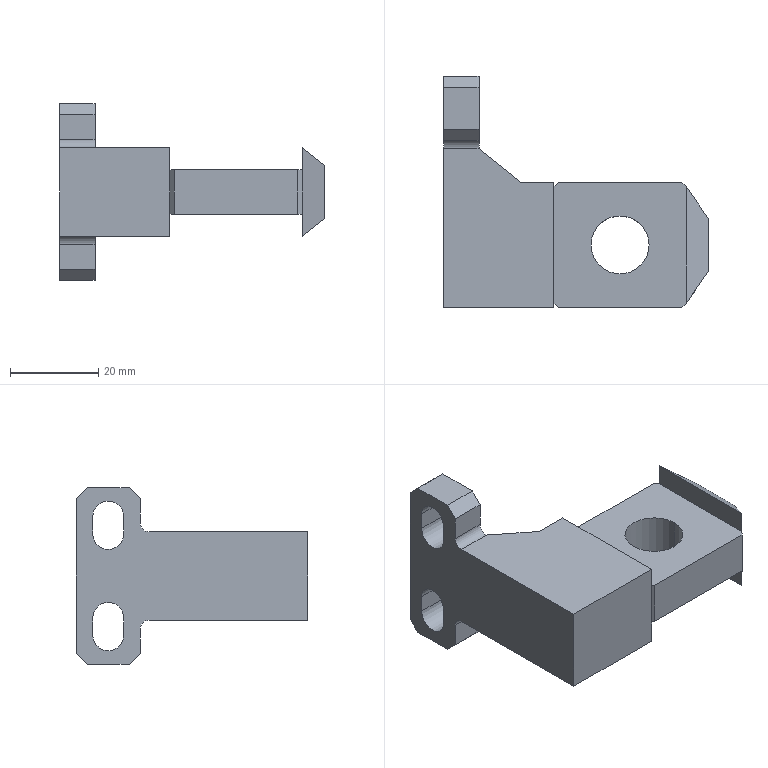Part | SolidWorks | features BaseBody 1 | 1 solid | 52 faces | box 60 x 52.5 x 40 mm | volume 28461 mm3 | plane 38 | cylinder 14 | commonest cylinder face diameters 7 x6 4 x2 6 x2 8 x2 13.157 x2
STEP:
#1=CARTESIAN_POINT('',(-6.579,0.,-5.));
#2=VERTEX_POINT('',#1);
#3=CARTESIAN_POINT('',(6.579,0.,-5.));
#4=VERTEX_POINT('',#3);
#5=CARTESIAN_POINT('',(0.,0.,-5.));
#6=DIRECTION('',(0.,0.,-1.));
#7=DIRECTION('',(-1.,0.,0.));
#8=AXIS2_PLACEMENT_3D('',#5,#6,#7);
#9=CIRCLE('',#8,6.579);
#10=EDGE_CURVE('',#2,#4,#9,.T.);
#11=ORIENTED_EDGE('',*,*,#10,.T.);
#12=CARTESIAN_POINT('',(6.579,0.,5.));
#13=VERTEX_POINT('',#12);
#14=CARTESIAN_POINT('',(6.579,0.,-5.));
#15=DIRECTION('',(0.,0.,1.));
#16=VECTOR('',#15,1000.);
#17=LINE('',#14,#16);
#18=EDGE_CURVE('',#4,#13,#17,.T.);
#19=ORIENTED_EDGE('',*,*,#18,.T.);
#20=CARTESIAN_POINT('',(-6.579,0.,5.));
#21=VERTEX_POINT('',#20);
#22=CARTESIAN_POINT('',(0.,0.,5.));
#23=DIRECTION('',(0.,0.,-1.));
#24=DIRECTION('',(-1.,0.,0.));
#25=AXIS2_PLACEMENT_3D('',#22,#23,#24);
#26=CIRCLE('',#25,6.579);
#27=EDGE_CURVE('',#21,#13,#26,.T.);
#28=ORIENTED_EDGE('',*,*,#27,.F.);
#29=CARTESIAN_POINT('',(-6.579,0.,-5.));
#30=DIRECTION('',(0.,0.,1.));
#31=VECTOR('',#30,1000.);
#32=LINE('',#29,#31);
#33=EDGE_CURVE('',#2,#21,#32,.T.);
#34=ORIENTED_EDGE('',*,*,#33,.F.);
#35=EDGE_LOOP('',(#11,#19,#28,#34));
#36=FACE_OUTER_BOUND('',#35,.T.);
#37=CARTESIAN_POINT('',(0.,0.,-5.));
#38=DIRECTION('',(0.,0.,1.));
#39=DIRECTION('',(-1.,0.,0.));
#40=AXIS2_PLACEMENT_3D('',#37,#38,#39);
#41=CYLINDRICAL_SURFACE('',#40,6.579);
#42=ADVANCED_FACE('',(#36),#41,.F.);
#43=CARTESIAN_POINT('',(20.,0.,-4.));
#44=VERTEX_POINT('',#43);
#45=CARTESIAN_POINT('',(20.,0.,4.));
#46=VERTEX_POINT('',#45);
#47=CARTESIAN_POINT('',(20.,0.,0.));
#48=DIRECTION('',(1.,0.,0.));
#49=DIRECTION('',(0.,0.,-1.));
#50=AXIS2_PLACEMENT_3D('',#47,#48,#49);
#51=CIRCLE('',#50,4.);
#52=EDGE_CURVE('',#44,#46,#51,.T.);
#53=ORIENTED_EDGE('',*,*,#52,.T.);
#54=CARTESIAN_POINT('',(18.,0.,4.));
#55=VERTEX_POINT('',#54);
#56=CARTESIAN_POINT('',(20.,0.,4.));
#57=DIRECTION('',(-1.,0.,0.));
#58=VECTOR('',#57,1000.);
#59=LINE('',#56,#58);
#60=EDGE_CURVE('',#46,#55,#59,.T.);
#61=ORIENTED_EDGE('',*,*,#60,.T.);
#62=CARTESIAN_POINT('',(18.,0.,-4.));
#63=VERTEX_POINT('',#62);
#64=CARTESIAN_POINT('',(18.,0.,0.));
#65=DIRECTION('',(1.,0.,0.));
#66=DIRECTION('',(0.,0.,-1.));
#67=AXIS2_PLACEMENT_3D('',#64,#65,#66);
#68=CIRCLE('',#67,4.);
#69=EDGE_CURVE('',#63,#55,#68,.T.);
#70=ORIENTED_EDGE('',*,*,#69,.F.);
#71=CARTESIAN_POINT('',(20.,0.,-4.));
#72=DIRECTION('',(-1.,0.,0.));
#73=VECTOR('',#72,1000.);
#74=LINE('',#71,#73);
#75=EDGE_CURVE('',#44,#63,#74,.T.);
#76=ORIENTED_EDGE('',*,*,#75,.F.);
#77=EDGE_LOOP('',(#53,#61,#70,#76));
#78=FACE_OUTER_BOUND('',#77,.T.);
#79=CARTESIAN_POINT('',(20.,0.,0.));
#80=DIRECTION('',(-1.,0.,0.));
#81=DIRECTION('',(0.,0.,-1.));
#82=AXIS2_PLACEMENT_3D('',#79,#80,#81);
#83=CYLINDRICAL_SURFACE('',#82,4.);
#84=ADVANCED_FACE('',(#78),#83,.F.);
#85=CARTESIAN_POINT('',(18.,0.,-3.));
#86=VERTEX_POINT('',#85);
#87=CARTESIAN_POINT('',(18.,0.,3.));
#88=VERTEX_POINT('',#87);
#89=CARTESIAN_POINT('',(18.,0.,0.));
#90=DIRECTION('',(1.,0.,0.));
#91=DIRECTION('',(0.,0.,-1.));
#92=AXIS2_PLACEMENT_3D('',#89,#90,#91);
#93=CIRCLE('',#92,3.);
#94=EDGE_CURVE('',#86,#88,#93,.T.);
#95=ORIENTED_EDGE('',*,*,#94,.T.);
#96=CARTESIAN_POINT('',(12.,0.,3.));
#97=VERTEX_POINT('',#96);
#98=CARTESIAN_POINT('',(20.,0.,3.));
#99=DIRECTION('',(-1.,0.,0.));
#100=VECTOR('',#99,1000.);
#101=LINE('',#98,#100);
#102=EDGE_CURVE('',#88,#97,#101,.T.);
#103=ORIENTED_EDGE('',*,*,#102,.T.);
#104=CARTESIAN_POINT('',(12.,0.,-3.));
#105=VERTEX_POINT('',#104);
#106=CARTESIAN_POINT('',(12.,0.,0.));
#107=DIRECTION('',(1.,0.,0.));
#108=DIRECTION('',(0.,0.,-1.));
#109=AXIS2_PLACEMENT_3D('',#106,#107,#108);
#110=CIRCLE('',#109,3.);
#111=EDGE_CURVE('',#105,#97,#110,.T.);
#112=ORIENTED_EDGE('',*,*,#111,.F.);
#113=CARTESIAN_POINT('',(20.,0.,-3.));
#114=DIRECTION('',(-1.,0.,0.));
#115=VECTOR('',#114,1000.);
#116=LINE('',#113,#115);
#117=EDGE_CURVE('',#86,#105,#116,.T.);
#118=ORIENTED_EDGE('',*,*,#117,.F.);
#119=EDGE_LOOP('',(#95,#103,#112,#118));
#120=FACE_OUTER_BOUND('',#119,.T.);
#121=CARTESIAN_POINT('',(20.,0.,0.));
#122=DIRECTION('',(-1.,0.,0.));
#123=DIRECTION('',(0.,0.,-1.));
#124=AXIS2_PLACEMENT_3D('',#121,#122,#123);
#125=CYLINDRICAL_SURFACE('',#124,3.);
#126=ADVANCED_FACE('',(#120),#125,.F.);
#127=CARTESIAN_POINT('',(-40.,31.,-6.));
#128=VERTEX_POINT('',#127);
#129=CARTESIAN_POINT('',(-40.,27.5,-9.5));
#130=VERTEX_POINT('',#129);
#131=CARTESIAN_POINT('',(-40.,31.,-9.5));
#132=DIRECTION('',(1.,0.,0.));
#133=DIRECTION('',(0.,0.,-1.));
#134=AXIS2_PLACEMENT_3D('',#131,#132,#133);
#135=CIRCLE('',#134,3.5);
#136=EDGE_CURVE('',#128,#130,#135,.T.);
#137=ORIENTED_EDGE('',*,*,#136,.F.);
#138=CARTESIAN_POINT('',(-32.,31.,-6.));
#139=VERTEX_POINT('',#138);
#140=CARTESIAN_POINT('',(-32.,31.,-6.));
#141=DIRECTION('',(1.,0.,0.));
#142=VECTOR('',#141,1000.);
#143=LINE('',#140,#142);
#144=EDGE_CURVE('',#128,#139,#143,.T.);
#145=ORIENTED_EDGE('',*,*,#144,.T.);
#146=CARTESIAN_POINT('',(-32.,27.5,-9.5));
#147=VERTEX_POINT('',#146);
#148=CARTESIAN_POINT('',(-32.,31.,-9.5));
#149=DIRECTION('',(1.,0.,0.));
#150=DIRECTION('',(0.,0.,-1.));
#151=AXIS2_PLACEMENT_3D('',#148,#149,#150);
#152=CIRCLE('',#151,3.5);
#153=EDGE_CURVE('',#139,#147,#152,.T.);
#154=ORIENTED_EDGE('',*,*,#153,.T.);
#155=CARTESIAN_POINT('',(-32.,27.5,-9.5));
#156=DIRECTION('',(-1.,0.,0.));
#157=VECTOR('',#156,1000.);
#158=LINE('',#155,#157);
#159=EDGE_CURVE('',#147,#130,#158,.T.);
#160=ORIENTED_EDGE('',*,*,#159,.T.);
#161=EDGE_LOOP('',(#137,#145,#154,#160));
#162=FACE_OUTER_BOUND('',#161,.T.);
#163=CARTESIAN_POINT('',(-32.,31.,-9.5));
#164=DIRECTION('',(1.,0.,0.));
#165=DIRECTION('',(0.,0.,1.));
#166=AXIS2_PLACEMENT_3D('',#163,#164,#165);
#167=CYLINDRICAL_SURFACE('',#166,3.5);
#168=ADVANCED_FACE('',(#162),#167,.F.);
#169=CARTESIAN_POINT('',(-40.,31.,17.));
#170=VERTEX_POINT('',#169);
#171=CARTESIAN_POINT('',(-40.,27.5,13.5));
#172=VERTEX_POINT('',#171);
#173=CARTESIAN_POINT('',(-40.,31.,13.5));
#174=DIRECTION('',(1.,0.,0.));
#175=DIRECTION('',(0.,0.,-1.));
#176=AXIS2_PLACEMENT_3D('',#173,#174,#175);
#177=CIRCLE('',#176,3.5);
#178=EDGE_CURVE('',#170,#172,#177,.T.);
#179=ORIENTED_EDGE('',*,*,#178,.F.);
#180=CARTESIAN_POINT('',(-32.,31.,17.));
#181=VERTEX_POINT('',#180);
#182=CARTESIAN_POINT('',(-32.,31.,17.));
#183=DIRECTION('',(1.,0.,0.));
#184=VECTOR('',#183,1000.);
#185=LINE('',#182,#184);
#186=EDGE_CURVE('',#170,#181,#185,.T.);
#187=ORIENTED_EDGE('',*,*,#186,.T.);
#188=CARTESIAN_POINT('',(-32.,27.5,13.5));
#189=VERTEX_POINT('',#188);
#190=CARTESIAN_POINT('',(-32.,31.,13.5));
#191=DIRECTION('',(1.,0.,0.));
#192=DIRECTION('',(0.,0.,-1.));
#193=AXIS2_PLACEMENT_3D('',#190,#191,#192);
#194=CIRCLE('',#193,3.5);
#195=EDGE_CURVE('',#181,#189,#194,.T.);
#196=ORIENTED_EDGE('',*,*,#195,.T.);
#197=CARTESIAN_POINT('',(-32.,27.5,13.5));
#198=DIRECTION('',(-1.,0.,0.));
#199=VECTOR('',#198,1000.);
#200=LINE('',#197,#199);
#201=EDGE_CURVE('',#189,#172,#200,.T.);
#202=ORIENTED_EDGE('',*,*,#201,.T.);
#203=EDGE_LOOP('',(#179,#187,#196,#202));
#204=FACE_OUTER_BOUND('',#203,.T.);
#205=CARTESIAN_POINT('',(-32.,31.,13.5));
#206=DIRECTION('',(1.,0.,0.));
#207=DIRECTION('',(0.,0.,1.));
#208=AXIS2_PLACEMENT_3D('',#205,#206,#207);
#209=CYLINDRICAL_SURFACE('',#208,3.5);
#210=ADVANCED_FACE('',(#204),#209,.F.);
#211=CARTESIAN_POINT('',(15.,13.25,-10.));
#212=VERTEX_POINT('',#211);
#213=CARTESIAN_POINT('',(20.,6.,-6.));
#214=VERTEX_POINT('',#213);
#215=CARTESIAN_POINT('',(23.42,1.041,-3.264));
#216=DIRECTION('',(0.5169,-0.7495,0.4135));
#217=VECTOR('',#216,1000.);
#218=LINE('',#215,#217);
#219=EDGE_CURVE('',#212,#214,#218,.T.);
#220=ORIENTED_EDGE('',*,*,#219,.T.);
#221=CARTESIAN_POINT('',(20.,-6.,-6.));
#222=VERTEX_POINT('',#221);
#223=CARTESIAN_POINT('',(20.,13.25,-6.));
#224=DIRECTION('',(0.,-1.,0.));
#225=VECTOR('',#224,1000.);
#226=LINE('',#223,#225);
#227=EDGE_CURVE('',#214,#222,#226,.T.);
#228=ORIENTED_EDGE('',*,*,#227,.T.);
#229=CARTESIAN_POINT('',(15.,-13.25,-10.));
#230=VERTEX_POINT('',#229);
#231=CARTESIAN_POINT('',(19.275,-7.051,-6.58));
#232=DIRECTION('',(-0.5169,-0.7495,-0.4135));
#233=VECTOR('',#232,1000.);
#234=LINE('',#231,#233);
#235=EDGE_CURVE('',#222,#230,#234,.T.);
#236=ORIENTED_EDGE('',*,*,#235,.T.);
#237=CARTESIAN_POINT('',(15.,13.25,-10.));
#238=DIRECTION('',(0.,-1.,0.));
#239=VECTOR('',#238,1000.);
#240=LINE('',#237,#239);
#241=EDGE_CURVE('',#212,#230,#240,.T.);
#242=ORIENTED_EDGE('',*,*,#241,.F.);
#243=EDGE_LOOP('',(#220,#228,#236,#242));
#244=FACE_OUTER_BOUND('',#243,.T.);
#245=CARTESIAN_POINT('',(15.,13.25,-10.));
#246=DIRECTION('',(0.6247,0.,-0.7809));
#247=DIRECTION('',(0.,-1.,0.));
#248=AXIS2_PLACEMENT_3D('',#245,#246,#247);
#249=PLANE('',#248);
#250=ADVANCED_FACE('',(#244),#249,.T.);
#251=CARTESIAN_POINT('',(20.,6.,6.));
#252=VERTEX_POINT('',#251);
#253=CARTESIAN_POINT('',(15.,13.25,10.));
#254=VERTEX_POINT('',#253);
#255=CARTESIAN_POINT('',(19.145,7.24,6.684));
#256=DIRECTION('',(-0.5169,0.7495,0.4135));
#257=VECTOR('',#256,1000.);
#258=LINE('',#255,#257);
#259=EDGE_CURVE('',#252,#254,#258,.T.);
#260=ORIENTED_EDGE('',*,*,#259,.T.);
#261=CARTESIAN_POINT('',(15.,-13.25,10.));
#262=VERTEX_POINT('',#261);
#263=CARTESIAN_POINT('',(15.,13.25,10.));
#264=DIRECTION('',(0.,-1.,0.));
#265=VECTOR('',#264,1000.);
#266=LINE('',#263,#265);
#267=EDGE_CURVE('',#254,#262,#266,.T.);
#268=ORIENTED_EDGE('',*,*,#267,.T.);
#269=CARTESIAN_POINT('',(20.,-6.,6.));
#270=VERTEX_POINT('',#269);
#271=CARTESIAN_POINT('',(15.,-13.25,10.));
#272=DIRECTION('',(0.5169,0.7495,-0.4135));
#273=VECTOR('',#272,1000.);
#274=LINE('',#271,#273);
#275=EDGE_CURVE('',#262,#270,#274,.T.);
#276=ORIENTED_EDGE('',*,*,#275,.T.);
#277=CARTESIAN_POINT('',(20.,13.25,6.));
#278=DIRECTION('',(0.,-1.,0.));
#279=VECTOR('',#278,1000.);
#280=LINE('',#277,#279);
#281=EDGE_CURVE('',#252,#270,#280,.T.);
#282=ORIENTED_EDGE('',*,*,#281,.F.);
#283=EDGE_LOOP('',(#260,#268,#276,#282));
#284=FACE_OUTER_BOUND('',#283,.T.);
#285=CARTESIAN_POINT('',(20.,13.25,6.));
#286=DIRECTION('',(0.6247,0.,0.7809));
#287=DIRECTION('',(0.,-1.,0.));
#288=AXIS2_PLACEMENT_3D('',#285,#286,#287);
#289=PLANE('',#288);
#290=ADVANCED_FACE('',(#284),#289,.T.);
#291=CARTESIAN_POINT('',(15.,-13.25,5.));
#292=VERTEX_POINT('',#291);
#293=CARTESIAN_POINT('',(15.,13.25,5.));
#294=VERTEX_POINT('',#293);
#295=CARTESIAN_POINT('',(15.,-13.25,5.));
#296=DIRECTION('',(0.,1.,0.));
#297=VECTOR('',#296,1000.);
#298=LINE('',#295,#297);
#299=EDGE_CURVE('',#292,#294,#298,.T.);
#300=ORIENTED_EDGE('',*,*,#299,.F.);
#301=CARTESIAN_POINT('',(15.,-13.25,10.));
#302=DIRECTION('',(0.,0.,-1.));
#303=VECTOR('',#302,1000.);
#304=LINE('',#301,#303);
#305=EDGE_CURVE('',#262,#292,#304,.T.);
#306=ORIENTED_EDGE('',*,*,#305,.F.);
#307=ORIENTED_EDGE('',*,*,#267,.F.);
#308=CARTESIAN_POINT('',(15.,13.25,10.));
#309=DIRECTION('',(0.,0.,-1.));
#310=VECTOR('',#309,1000.);
#311=LINE('',#308,#310);
#312=EDGE_CURVE('',#254,#294,#311,.T.);
#313=ORIENTED_EDGE('',*,*,#312,.T.);
#314=EDGE_LOOP('',(#300,#306,#307,#313));
#315=FACE_OUTER_BOUND('',#314,.T.);
#316=CARTESIAN_POINT('',(15.,13.25,10.));
#317=DIRECTION('',(1.,0.,0.));
#318=DIRECTION('',(0.,1.,0.));
#319=AXIS2_PLACEMENT_3D('',#316,#317,#318);
#320=PLANE('',#319);
#321=ADVANCED_FACE('',(#315),#320,.F.);
#322=ORIENTED_EDGE('',*,*,#259,.F.);
#323=CARTESIAN_POINT('',(20.,6.,10.));
#324=DIRECTION('',(0.,0.,-1.));
#325=VECTOR('',#324,1000.);
#326=LINE('',#323,#325);
#327=EDGE_CURVE('',#252,#214,#326,.T.);
#328=ORIENTED_EDGE('',*,*,#327,.T.);
#329=ORIENTED_EDGE('',*,*,#219,.F.);
#330=CARTESIAN_POINT('',(15.,13.25,-5.));
#331=VERTEX_POINT('',#330);
#332=CARTESIAN_POINT('',(15.,13.25,10.));
#333=DIRECTION('',(0.,0.,-1.));
#334=VECTOR('',#333,1000.);
#335=LINE('',#332,#334);
#336=EDGE_CURVE('',#331,#212,#335,.T.);
#337=ORIENTED_EDGE('',*,*,#336,.F.);
#338=CARTESIAN_POINT('',(15.,13.25,5.));
#339=DIRECTION('',(0.,0.,-1.));
#340=VECTOR('',#339,1000.);
#341=LINE('',#338,#340);
#342=EDGE_CURVE('',#294,#331,#341,.T.);
#343=ORIENTED_EDGE('',*,*,#342,.F.);
#344=ORIENTED_EDGE('',*,*,#312,.F.);
#345=EDGE_LOOP('',(#322,#328,#329,#337,#343,#344));
#346=FACE_OUTER_BOUND('',#345,.T.);
#347=CARTESIAN_POINT('',(20.,6.,10.));
#348=DIRECTION('',(-0.8232,-0.5677,0.));
#349=DIRECTION('',(-0.5677,0.8232,0.));
#350=AXIS2_PLACEMENT_3D('',#347,#348,#349);
#351=PLANE('',#350);
#352=ADVANCED_FACE('',(#346),#351,.F.);
#353=ORIENTED_EDGE('',*,*,#275,.F.);
#354=ORIENTED_EDGE('',*,*,#305,.T.);
#355=CARTESIAN_POINT('',(15.,-13.25,-5.));
#356=VERTEX_POINT('',#355);
#357=CARTESIAN_POINT('',(15.,-13.25,5.));
#358=DIRECTION('',(0.,0.,-1.));
#359=VECTOR('',#358,1000.);
#360=LINE('',#357,#359);
#361=EDGE_CURVE('',#292,#356,#360,.T.);
#362=ORIENTED_EDGE('',*,*,#361,.T.);
#363=CARTESIAN_POINT('',(15.,-13.25,10.));
#364=DIRECTION('',(0.,0.,-1.));
#365=VECTOR('',#364,1000.);
#366=LINE('',#363,#365);
#367=EDGE_CURVE('',#356,#230,#366,.T.);
#368=ORIENTED_EDGE('',*,*,#367,.T.);
#369=ORIENTED_EDGE('',*,*,#235,.F.);
#370=CARTESIAN_POINT('',(20.,-6.,10.));
#371=DIRECTION('',(0.,0.,-1.));
#372=VECTOR('',#371,1000.);
#373=LINE('',#370,#372);
#374=EDGE_CURVE('',#270,#222,#373,.T.);
#375=ORIENTED_EDGE('',*,*,#374,.F.);
#376=EDGE_LOOP('',(#353,#354,#362,#368,#369,#375));
#377=FACE_OUTER_BOUND('',#376,.T.);
#378=CARTESIAN_POINT('',(15.,-13.25,10.));
#379=DIRECTION('',(-0.8232,0.5677,0.));
#380=DIRECTION('',(0.,0.,1.));
#381=AXIS2_PLACEMENT_3D('',#378,#379,#380);
#382=PLANE('',#381);
#383=ADVANCED_FACE('',(#377),#382,.F.);
#384=ORIENTED_EDGE('',*,*,#27,.T.);
#385=CARTESIAN_POINT('',(0.,0.,5.));
#386=DIRECTION('',(0.,0.,-1.));
#387=DIRECTION('',(-1.,0.,0.));
#388=AXIS2_PLACEMENT_3D('',#385,#386,#387);
#389=CIRCLE('',#388,6.579);
#390=EDGE_CURVE('',#13,#21,#389,.T.);
#391=ORIENTED_EDGE('',*,*,#390,.T.);
#392=EDGE_LOOP('',(#384,#391));
#393=FACE_BOUND('',#392,.T.);
#394=CARTESIAN_POINT('',(-14.,14.25,5.));
#395=VERTEX_POINT('',#394);
#396=CARTESIAN_POINT('',(-15.,13.25,5.));
#397=VERTEX_POINT('',#396);
#398=CARTESIAN_POINT('',(-14.,14.25,5.));
#399=DIRECTION('',(-0.7071,-0.7071,0.));
#400=VECTOR('',#399,1000.);
#401=LINE('',#398,#400);
#402=EDGE_CURVE('',#395,#397,#401,.T.);
#403=ORIENTED_EDGE('',*,*,#402,.T.);
#404=CARTESIAN_POINT('',(-15.,-13.25,5.));
#405=VERTEX_POINT('',#404);
#406=CARTESIAN_POINT('',(-15.,13.25,5.));
#407=DIRECTION('',(0.,-1.,0.));
#408=VECTOR('',#407,1000.);
#409=LINE('',#406,#408);
#410=EDGE_CURVE('',#397,#405,#409,.T.);
#411=ORIENTED_EDGE('',*,*,#410,.T.);
#412=CARTESIAN_POINT('',(-14.,-14.25,5.));
#413=VERTEX_POINT('',#412);
#414=CARTESIAN_POINT('',(-15.,-13.25,5.));
#415=DIRECTION('',(0.7071,-0.7071,0.));
#416=VECTOR('',#415,1000.);
#417=LINE('',#414,#416);
#418=EDGE_CURVE('',#405,#413,#417,.T.);
#419=ORIENTED_EDGE('',*,*,#418,.T.);
#420=CARTESIAN_POINT('',(14.,-14.25,5.));
#421=VERTEX_POINT('',#420);
#422=CARTESIAN_POINT('',(-14.,-14.25,5.));
#423=DIRECTION('',(1.,0.,0.));
#424=VECTOR('',#423,1000.);
#425=LINE('',#422,#424);
#426=EDGE_CURVE('',#413,#421,#425,.T.);
#427=ORIENTED_EDGE('',*,*,#426,.T.);
#428=CARTESIAN_POINT('',(14.,-14.25,5.));
#429=DIRECTION('',(0.7071,0.7071,0.));
#430=VECTOR('',#429,1000.);
#431=LINE('',#428,#430);
#432=EDGE_CURVE('',#421,#292,#431,.T.);
#433=ORIENTED_EDGE('',*,*,#432,.T.);
#434=ORIENTED_EDGE('',*,*,#299,.T.);
#435=CARTESIAN_POINT('',(14.,14.25,5.));
#436=VERTEX_POINT('',#435);
#437=CARTESIAN_POINT('',(15.,13.25,5.));
#438=DIRECTION('',(-0.7071,0.7071,0.));
#439=VECTOR('',#438,1000.);
#440=LINE('',#437,#439);
#441=EDGE_CURVE('',#294,#436,#440,.T.);
#442=ORIENTED_EDGE('',*,*,#441,.T.);
#443=CARTESIAN_POINT('',(14.,14.25,5.));
#444=DIRECTION('',(-1.,0.,0.));
#445=VECTOR('',#444,1000.);
#446=LINE('',#443,#445);
#447=EDGE_CURVE('',#436,#395,#446,.T.);
#448=ORIENTED_EDGE('',*,*,#447,.T.);
#449=EDGE_LOOP('',(#403,#411,#419,#427,#433,#434,#442,#448));
#450=FACE_OUTER_BOUND('',#449,.T.);
#451=CARTESIAN_POINT('',(0.,0.,5.));
#452=DIRECTION('',(0.,0.,1.));
#453=DIRECTION('',(1.,0.,0.));
#454=AXIS2_PLACEMENT_3D('',#451,#452,#453);
#455=PLANE('',#454);
#456=ADVANCED_FACE('',(#393,#450),#455,.T.);
#457=ORIENTED_EDGE('',*,*,#10,.F.);
#458=CARTESIAN_POINT('',(0.,0.,-5.));
#459=DIRECTION('',(0.,0.,-1.));
#460=DIRECTION('',(-1.,0.,0.));
#461=AXIS2_PLACEMENT_3D('',#458,#459,#460);
#462=CIRCLE('',#461,6.579);
#463=EDGE_CURVE('',#4,#2,#462,.T.);
#464=ORIENTED_EDGE('',*,*,#463,.F.);
#465=EDGE_LOOP('',(#457,#464));
#466=FACE_BOUND('',#465,.T.);
#467=CARTESIAN_POINT('',(-14.,14.25,-5.));
#468=VERTEX_POINT('',#467);
#469=CARTESIAN_POINT('',(-15.,13.25,-5.));
#470=VERTEX_POINT('',#469);
#471=CARTESIAN_POINT('',(-14.,14.25,-5.));
#472=DIRECTION('',(-0.7071,-0.7071,0.));
#473=VECTOR('',#472,1000.);
#474=LINE('',#471,#473);
#475=EDGE_CURVE('',#468,#470,#474,.T.);
#476=ORIENTED_EDGE('',*,*,#475,.F.);
#477=CARTESIAN_POINT('',(14.,14.25,-5.));
#478=VERTEX_POINT('',#477);
#479=CARTESIAN_POINT('',(14.,14.25,-5.));
#480=DIRECTION('',(-1.,0.,0.));
#481=VECTOR('',#480,1000.);
#482=LINE('',#479,#481);
#483=EDGE_CURVE('',#478,#468,#482,.T.);
#484=ORIENTED_EDGE('',*,*,#483,.F.);
#485=CARTESIAN_POINT('',(15.,13.25,-5.));
#486=DIRECTION('',(-0.7071,0.7071,0.));
#487=VECTOR('',#486,1000.);
#488=LINE('',#485,#487);
#489=EDGE_CURVE('',#331,#478,#488,.T.);
#490=ORIENTED_EDGE('',*,*,#489,.F.);
#491=CARTESIAN_POINT('',(15.,-13.25,-5.));
#492=DIRECTION('',(0.,1.,0.));
#493=VECTOR('',#492,1000.);
#494=LINE('',#491,#493);
#495=EDGE_CURVE('',#356,#331,#494,.T.);
#496=ORIENTED_EDGE('',*,*,#495,.F.);
#497=CARTESIAN_POINT('',(14.,-14.25,-5.));
#498=VERTEX_POINT('',#497);
#499=CARTESIAN_POINT('',(14.,-14.25,-5.));
#500=DIRECTION('',(0.7071,0.7071,0.));
#501=VECTOR('',#500,1000.);
#502=LINE('',#499,#501);
#503=EDGE_CURVE('',#498,#356,#502,.T.);
#504=ORIENTED_EDGE('',*,*,#503,.F.);
#505=CARTESIAN_POINT('',(-14.,-14.25,-5.));
#506=VERTEX_POINT('',#505);
#507=CARTESIAN_POINT('',(-14.,-14.25,-5.));
#508=DIRECTION('',(1.,0.,0.));
#509=VECTOR('',#508,1000.);
#510=LINE('',#507,#509);
#511=EDGE_CURVE('',#506,#498,#510,.T.);
#512=ORIENTED_EDGE('',*,*,#511,.F.);
#513=CARTESIAN_POINT('',(-15.,-13.25,-5.));
#514=VERTEX_POINT('',#513);
#515=CARTESIAN_POINT('',(-15.,-13.25,-5.));
#516=DIRECTION('',(0.7071,-0.7071,0.));
#517=VECTOR('',#516,1000.);
#518=LINE('',#515,#517);
#519=EDGE_CURVE('',#514,#506,#518,.T.);
#520=ORIENTED_EDGE('',*,*,#519,.F.);
#521=CARTESIAN_POINT('',(-15.,13.25,-5.));
#522=DIRECTION('',(0.,-1.,0.));
#523=VECTOR('',#522,1000.);
#524=LINE('',#521,#523);
#525=EDGE_CURVE('',#470,#514,#524,.T.);
#526=ORIENTED_EDGE('',*,*,#525,.F.);
#527=EDGE_LOOP('',(#476,#484,#490,#496,#504,#512,#520,#526));
#528=FACE_OUTER_BOUND('',#527,.T.);
#529=CARTESIAN_POINT('',(0.,0.,-5.));
#530=DIRECTION('',(0.,0.,1.));
#531=DIRECTION('',(1.,0.,0.));
#532=AXIS2_PLACEMENT_3D('',#529,#530,#531);
#533=PLANE('',#532);
#534=ADVANCED_FACE('',(#466,#528),#533,.F.);
#535=ORIENTED_EDGE('',*,*,#483,.T.);
#536=CARTESIAN_POINT('',(-14.,14.25,5.));
#537=DIRECTION('',(0.,0.,-1.));
#538=VECTOR('',#537,1000.);
#539=LINE('',#536,#538);
#540=EDGE_CURVE('',#395,#468,#539,.T.);
#541=ORIENTED_EDGE('',*,*,#540,.F.);
#542=ORIENTED_EDGE('',*,*,#447,.F.);
#543=CARTESIAN_POINT('',(14.,14.25,5.));
#544=DIRECTION('',(0.,0.,-1.));
#545=VECTOR('',#544,1000.);
#546=LINE('',#543,#545);
#547=EDGE_CURVE('',#436,#478,#546,.T.);
#548=ORIENTED_EDGE('',*,*,#547,.T.);
#549=EDGE_LOOP('',(#535,#541,#542,#548));
#550=FACE_OUTER_BOUND('',#549,.T.);
#551=CARTESIAN_POINT('',(14.,14.25,5.));
#552=DIRECTION('',(0.,-1.,0.));
#553=DIRECTION('',(0.,0.,-1.));
#554=AXIS2_PLACEMENT_3D('',#551,#552,#553);
#555=PLANE('',#554);
#556=ADVANCED_FACE('',(#550),#555,.F.);
#557=ORIENTED_EDGE('',*,*,#489,.T.);
#558=ORIENTED_EDGE('',*,*,#547,.F.);
#559=ORIENTED_EDGE('',*,*,#441,.F.);
#560=ORIENTED_EDGE('',*,*,#342,.T.);
#561=EDGE_LOOP('',(#557,#558,#559,#560));
#562=FACE_OUTER_BOUND('',#561,.T.);
#563=CARTESIAN_POINT('',(15.,13.25,5.));
#564=DIRECTION('',(-0.7071,-0.7071,0.));
#565=DIRECTION('',(-0.7071,0.7071,0.));
#566=AXIS2_PLACEMENT_3D('',#563,#564,#565);
#567=PLANE('',#566);
#568=ADVANCED_FACE('',(#562),#567,.F.);
#569=ORIENTED_EDGE('',*,*,#503,.T.);
#570=ORIENTED_EDGE('',*,*,#361,.F.);
#571=ORIENTED_EDGE('',*,*,#432,.F.);
#572=CARTESIAN_POINT('',(14.,-14.25,5.));
#573=DIRECTION('',(0.,0.,-1.));
#574=VECTOR('',#573,1000.);
#575=LINE('',#572,#574);
#576=EDGE_CURVE('',#421,#498,#575,.T.);
#577=ORIENTED_EDGE('',*,*,#576,.T.);
#578=EDGE_LOOP('',(#569,#570,#571,#577));
#579=FACE_OUTER_BOUND('',#578,.T.);
#580=CARTESIAN_POINT('',(14.,-14.25,5.));
#581=DIRECTION('',(-0.7071,0.7071,0.));
#582=DIRECTION('',(0.,0.,1.));
#583=AXIS2_PLACEMENT_3D('',#580,#581,#582);
#584=PLANE('',#583);
#585=ADVANCED_FACE('',(#579),#584,.F.);
#586=ORIENTED_EDGE('',*,*,#511,.T.);
#587=ORIENTED_EDGE('',*,*,#576,.F.);
#588=ORIENTED_EDGE('',*,*,#426,.F.);
#589=CARTESIAN_POINT('',(-14.,-14.25,5.));
#590=DIRECTION('',(0.,0.,-1.));
#591=VECTOR('',#590,1000.);
#592=LINE('',#589,#591);
#593=EDGE_CURVE('',#413,#506,#592,.T.);
#594=ORIENTED_EDGE('',*,*,#593,.T.);
#595=EDGE_LOOP('',(#586,#587,#588,#594));
#596=FACE_OUTER_BOUND('',#595,.T.);
#597=CARTESIAN_POINT('',(-14.,-14.25,5.));
#598=DIRECTION('',(0.,1.,0.));
#599=DIRECTION('',(1.,0.,0.));
#600=AXIS2_PLACEMENT_3D('',#597,#598,#599);
#601=PLANE('',#600);
#602=ADVANCED_FACE('',(#596),#601,.F.);
#603=ORIENTED_EDGE('',*,*,#519,.T.);
#604=ORIENTED_EDGE('',*,*,#593,.F.);
#605=ORIENTED_EDGE('',*,*,#418,.F.);
#606=CARTESIAN_POINT('',(-15.,-13.25,5.));
#607=DIRECTION('',(0.,0.,-1.));
#608=VECTOR('',#607,1000.);
#609=LINE('',#606,#608);
#610=EDGE_CURVE('',#405,#514,#609,.T.);
#611=ORIENTED_EDGE('',*,*,#610,.T.);
#612=EDGE_LOOP('',(#603,#604,#605,#611));
#613=FACE_OUTER_BOUND('',#612,.T.);
#614=CARTESIAN_POINT('',(-15.,-13.25,5.));
#615=DIRECTION('',(0.7071,0.7071,0.));
#616=DIRECTION('',(0.,0.,-1.));
#617=AXIS2_PLACEMENT_3D('',#614,#615,#616);
#618=PLANE('',#617);
#619=ADVANCED_FACE('',(#613),#618,.F.);
#620=ORIENTED_EDGE('',*,*,#475,.T.);
#621=CARTESIAN_POINT('',(-15.,13.25,5.));
#622=DIRECTION('',(0.,0.,-1.));
#623=VECTOR('',#622,1000.);
#624=LINE('',#621,#623);
#625=EDGE_CURVE('',#397,#470,#624,.T.);
#626=ORIENTED_EDGE('',*,*,#625,.F.);
#627=ORIENTED_EDGE('',*,*,#402,.F.);
#628=ORIENTED_EDGE('',*,*,#540,.T.);
#629=EDGE_LOOP('',(#620,#626,#627,#628));
#630=FACE_OUTER_BOUND('',#629,.T.);
#631=CARTESIAN_POINT('',(-14.,14.25,5.));
#632=DIRECTION('',(0.7071,-0.7071,0.));
#633=DIRECTION('',(0.,0.,-1.));
#634=AXIS2_PLACEMENT_3D('',#631,#632,#633);
#635=PLANE('',#634);
#636=ADVANCED_FACE('',(#630),#635,.F.);
#637=ORIENTED_EDGE('',*,*,#52,.F.);
#638=CARTESIAN_POINT('',(20.,0.,0.));
#639=DIRECTION('',(1.,0.,0.));
#640=DIRECTION('',(0.,0.,-1.));
#641=AXIS2_PLACEMENT_3D('',#638,#639,#640);
#642=CIRCLE('',#641,4.);
#643=EDGE_CURVE('',#46,#44,#642,.T.);
#644=ORIENTED_EDGE('',*,*,#643,.F.);
#645=EDGE_LOOP('',(#637,#644));
#646=FACE_BOUND('',#645,.T.);
#647=ORIENTED_EDGE('',*,*,#281,.T.);
#648=ORIENTED_EDGE('',*,*,#374,.T.);
#649=ORIENTED_EDGE('',*,*,#227,.F.);
#650=ORIENTED_EDGE('',*,*,#327,.F.);
#651=EDGE_LOOP('',(#647,#648,#649,#650));
#652=FACE_OUTER_BOUND('',#651,.T.);
#653=CARTESIAN_POINT('',(20.,-6.,10.));
#654=DIRECTION('',(-1.,0.,0.));
#655=DIRECTION('',(0.,0.,1.));
#656=AXIS2_PLACEMENT_3D('',#653,#654,#655);
#657=PLANE('',#656);
#658=ADVANCED_FACE('',(#646,#652),#657,.F.);
#659=ORIENTED_EDGE('',*,*,#94,.F.);
#660=CARTESIAN_POINT('',(18.,0.,0.));
#661=DIRECTION('',(1.,0.,0.));
#662=DIRECTION('',(0.,0.,-1.));
#663=AXIS2_PLACEMENT_3D('',#660,#661,#662);
#664=CIRCLE('',#663,3.);
#665=EDGE_CURVE('',#88,#86,#664,.T.);
#666=ORIENTED_EDGE('',*,*,#665,.F.);
#667=EDGE_LOOP('',(#659,#666));
#668=FACE_BOUND('',#667,.T.);
#669=ORIENTED_EDGE('',*,*,#69,.T.);
#670=CARTESIAN_POINT('',(18.,0.,0.));
#671=DIRECTION('',(1.,0.,0.));
#672=DIRECTION('',(0.,0.,-1.));
#673=AXIS2_PLACEMENT_3D('',#670,#671,#672);
#674=CIRCLE('',#673,4.);
#675=EDGE_CURVE('',#55,#63,#674,.T.);
#676=ORIENTED_EDGE('',*,*,#675,.T.);
#677=EDGE_LOOP('',(#669,#676));
#678=FACE_OUTER_BOUND('',#677,.T.);
#679=CARTESIAN_POINT('',(18.,3.,0.));
#680=DIRECTION('',(1.,0.,0.));
#681=DIRECTION('',(0.,1.,0.));
#682=AXIS2_PLACEMENT_3D('',#679,#680,#681);
#683=PLANE('',#682);
#684=ADVANCED_FACE('',(#668,#678),#683,.T.);
#685=ORIENTED_EDGE('',*,*,#111,.T.);
#686=CARTESIAN_POINT('',(12.,0.,0.));
#687=DIRECTION('',(1.,0.,0.));
#688=DIRECTION('',(0.,0.,-1.));
#689=AXIS2_PLACEMENT_3D('',#686,#687,#688);
#690=CIRCLE('',#689,3.);
#691=EDGE_CURVE('',#97,#105,#690,.T.);
#692=ORIENTED_EDGE('',*,*,#691,.T.);
#693=EDGE_LOOP('',(#685,#692));
#694=FACE_OUTER_BOUND('',#693,.T.);
#695=CARTESIAN_POINT('',(12.,0.,0.));
#696=DIRECTION('',(1.,0.,0.));
#697=DIRECTION('',(0.,1.,0.));
#698=AXIS2_PLACEMENT_3D('',#695,#696,#697);
#699=PLANE('',#698);
#700=ADVANCED_FACE('',(#694),#699,.T.);
#701=CARTESIAN_POINT('',(-40.,34.5,9.5));
#702=VERTEX_POINT('',#701);
#703=CARTESIAN_POINT('',(-40.,34.5,13.5));
#704=VERTEX_POINT('',#703);
#705=CARTESIAN_POINT('',(-40.,34.5,9.5));
#706=DIRECTION('',(0.,0.,1.));
#707=VECTOR('',#706,1000.);
#708=LINE('',#705,#707);
#709=EDGE_CURVE('',#702,#704,#708,.T.);
#710=ORIENTED_EDGE('',*,*,#709,.T.);
#711=CARTESIAN_POINT('',(-40.,31.,13.5));
#712=DIRECTION('',(1.,0.,0.));
#713=DIRECTION('',(0.,0.,-1.));
#714=AXIS2_PLACEMENT_3D('',#711,#712,#713);
#715=CIRCLE('',#714,3.5);
#716=EDGE_CURVE('',#704,#170,#715,.T.);
#717=ORIENTED_EDGE('',*,*,#716,.T.);
#718=ORIENTED_EDGE('',*,*,#178,.T.);
#719=CARTESIAN_POINT('',(-40.,27.5,9.5));
#720=VERTEX_POINT('',#719);
#721=CARTESIAN_POINT('',(-40.,27.5,13.5));
#722=DIRECTION('',(0.,0.,-1.));
#723=VECTOR('',#722,1000.);
#724=LINE('',#721,#723);
#725=EDGE_CURVE('',#172,#720,#724,.T.);
#726=ORIENTED_EDGE('',*,*,#725,.T.);
#727=CARTESIAN_POINT('',(-40.,31.,9.5));
#728=DIRECTION('',(1.,0.,0.));
#729=DIRECTION('',(0.,0.,-1.));
#730=AXIS2_PLACEMENT_3D('',#727,#728,#729);
#731=CIRCLE('',#730,3.5);
#732=EDGE_CURVE('',#720,#702,#731,.T.);
#733=ORIENTED_EDGE('',*,*,#732,.T.);
#734=EDGE_LOOP('',(#710,#717,#718,#726,#733));
#735=FACE_BOUND('',#734,.T.);
#736=CARTESIAN_POINT('',(-40.,34.5,-13.5));
#737=VERTEX_POINT('',#736);
#738=CARTESIAN_POINT('',(-40.,34.5,-9.5));
#739=VERTEX_POINT('',#738);
#740=CARTESIAN_POINT('',(-40.,34.5,-13.5));
#741=DIRECTION('',(0.,0.,1.));
#742=VECTOR('',#741,1000.);
#743=LINE('',#740,#742);
#744=EDGE_CURVE('',#737,#739,#743,.T.);
#745=ORIENTED_EDGE('',*,*,#744,.T.);
#746=CARTESIAN_POINT('',(-40.,31.,-9.5));
#747=DIRECTION('',(1.,0.,0.));
#748=DIRECTION('',(0.,0.,-1.));
#749=AXIS2_PLACEMENT_3D('',#746,#747,#748);
#750=CIRCLE('',#749,3.5);
#751=EDGE_CURVE('',#739,#128,#750,.T.);
#752=ORIENTED_EDGE('',*,*,#751,.T.);
#753=ORIENTED_EDGE('',*,*,#136,.T.);
#754=CARTESIAN_POINT('',(-40.,27.5,-13.5));
#755=VERTEX_POINT('',#754);
#756=CARTESIAN_POINT('',(-40.,27.5,-9.5));
#757=DIRECTION('',(0.,0.,-1.));
#758=VECTOR('',#757,1000.);
#759=LINE('',#756,#758);
#760=EDGE_CURVE('',#130,#755,#759,.T.);
#761=ORIENTED_EDGE('',*,*,#760,.T.);
#762=CARTESIAN_POINT('',(-40.,31.,-13.5));
#763=DIRECTION('',(1.,0.,0.));
#764=DIRECTION('',(0.,0.,-1.));
#765=AXIS2_PLACEMENT_3D('',#762,#763,#764);
#766=CIRCLE('',#765,3.5);
#767=EDGE_CURVE('',#755,#737,#766,.T.);
#768=ORIENTED_EDGE('',*,*,#767,.T.);
#769=EDGE_LOOP('',(#745,#752,#753,#761,#768));
#770=FACE_BOUND('',#769,.T.);
#771=CARTESIAN_POINT('',(-40.,21.75,-10.));
#772=VERTEX_POINT('',#771);
#773=CARTESIAN_POINT('',(-40.,-14.25,-10.));
#774=VERTEX_POINT('',#773);
#775=CARTESIAN_POINT('',(-40.,21.75,-10.));
#776=DIRECTION('',(0.,-1.,0.));
#777=VECTOR('',#776,1000.);
#778=LINE('',#775,#777);
#779=EDGE_CURVE('',#772,#774,#778,.T.);
#780=ORIENTED_EDGE('',*,*,#779,.T.);
#781=CARTESIAN_POINT('',(-40.,-14.25,10.));
#782=VERTEX_POINT('',#781);
#783=CARTESIAN_POINT('',(-40.,-14.25,10.));
#784=DIRECTION('',(0.,0.,-1.));
#785=VECTOR('',#784,1000.);
#786=LINE('',#783,#785);
#787=EDGE_CURVE('',#782,#774,#786,.T.);
#788=ORIENTED_EDGE('',*,*,#787,.F.);
#789=CARTESIAN_POINT('',(-40.,21.75,10.));
#790=VERTEX_POINT('',#789);
#791=CARTESIAN_POINT('',(-40.,21.75,10.));
#792=DIRECTION('',(0.,-1.,0.));
#793=VECTOR('',#792,1000.);
#794=LINE('',#791,#793);
#795=EDGE_CURVE('',#790,#782,#794,.T.);
#796=ORIENTED_EDGE('',*,*,#795,.F.);
#797=CARTESIAN_POINT('',(-40.,23.75,12.));
#798=VERTEX_POINT('',#797);
#799=CARTESIAN_POINT('',(-40.,21.75,12.));
#800=DIRECTION('',(1.,0.,0.));
#801=DIRECTION('',(0.,0.,-1.));
#802=AXIS2_PLACEMENT_3D('',#799,#800,#801);
#803=CIRCLE('',#802,2.);
#804=EDGE_CURVE('',#790,#798,#803,.T.);
#805=ORIENTED_EDGE('',*,*,#804,.T.);
#806=CARTESIAN_POINT('',(-40.,23.75,17.5));
#807=VERTEX_POINT('',#806);
#808=CARTESIAN_POINT('',(-40.,23.75,17.5));
#809=DIRECTION('',(0.,0.,-1.));
#810=VECTOR('',#809,1000.);
#811=LINE('',#808,#810);
#812=EDGE_CURVE('',#807,#798,#811,.T.);
#813=ORIENTED_EDGE('',*,*,#812,.F.);
#814=CARTESIAN_POINT('',(-40.,26.25,20.));
#815=VERTEX_POINT('',#814);
#816=CARTESIAN_POINT('',(-40.,26.25,20.));
#817=DIRECTION('',(0.,-0.7071,-0.7071));
#818=VECTOR('',#817,1000.);
#819=LINE('',#816,#818);
#820=EDGE_CURVE('',#815,#807,#819,.T.);
#821=ORIENTED_EDGE('',*,*,#820,.F.);
#822=CARTESIAN_POINT('',(-40.,35.75,20.));
#823=VERTEX_POINT('',#822);
#824=CARTESIAN_POINT('',(-40.,35.75,20.));
#825=DIRECTION('',(0.,-1.,0.));
#826=VECTOR('',#825,1000.);
#827=LINE('',#824,#826);
#828=EDGE_CURVE('',#823,#815,#827,.T.);
#829=ORIENTED_EDGE('',*,*,#828,.F.);
#830=CARTESIAN_POINT('',(-40.,38.25,17.5));
#831=VERTEX_POINT('',#830);
#832=CARTESIAN_POINT('',(-40.,38.25,17.5));
#833=DIRECTION('',(0.,-0.7071,0.7071));
#834=VECTOR('',#833,1000.);
#835=LINE('',#832,#834);
#836=EDGE_CURVE('',#831,#823,#835,.T.);
#837=ORIENTED_EDGE('',*,*,#836,.F.);
#838=CARTESIAN_POINT('',(-40.,38.25,-17.5));
#839=VERTEX_POINT('',#838);
#840=CARTESIAN_POINT('',(-40.,38.25,-17.5));
#841=DIRECTION('',(0.,0.,1.));
#842=VECTOR('',#841,1000.);
#843=LINE('',#840,#842);
#844=EDGE_CURVE('',#839,#831,#843,.T.);
#845=ORIENTED_EDGE('',*,*,#844,.F.);
#846=CARTESIAN_POINT('',(-40.,35.75,-20.));
#847=VERTEX_POINT('',#846);
#848=CARTESIAN_POINT('',(-40.,35.75,-20.));
#849=DIRECTION('',(0.,0.7071,0.7071));
#850=VECTOR('',#849,1000.);
#851=LINE('',#848,#850);
#852=EDGE_CURVE('',#847,#839,#851,.T.);
#853=ORIENTED_EDGE('',*,*,#852,.F.);
#854=CARTESIAN_POINT('',(-40.,26.25,-20.));
#855=VERTEX_POINT('',#854);
#856=CARTESIAN_POINT('',(-40.,26.25,-20.));
#857=DIRECTION('',(0.,1.,0.));
#858=VECTOR('',#857,1000.);
#859=LINE('',#856,#858);
#860=EDGE_CURVE('',#855,#847,#859,.T.);
#861=ORIENTED_EDGE('',*,*,#860,.F.);
#862=CARTESIAN_POINT('',(-40.,23.75,-17.5));
#863=VERTEX_POINT('',#862);
#864=CARTESIAN_POINT('',(-40.,23.75,-17.5));
#865=DIRECTION('',(0.,0.7071,-0.7071));
#866=VECTOR('',#865,1000.);
#867=LINE('',#864,#866);
#868=EDGE_CURVE('',#863,#855,#867,.T.);
#869=ORIENTED_EDGE('',*,*,#868,.F.);
#870=CARTESIAN_POINT('',(-40.,23.75,-12.));
#871=VERTEX_POINT('',#870);
#872=CARTESIAN_POINT('',(-40.,23.75,-12.));
#873=DIRECTION('',(0.,0.,-1.));
#874=VECTOR('',#873,1000.);
#875=LINE('',#872,#874);
#876=EDGE_CURVE('',#871,#863,#875,.T.);
#877=ORIENTED_EDGE('',*,*,#876,.F.);
#878=CARTESIAN_POINT('',(-40.,21.75,-12.));
#879=DIRECTION('',(1.,0.,0.));
#880=DIRECTION('',(0.,0.,-1.));
#881=AXIS2_PLACEMENT_3D('',#878,#879,#880);
#882=CIRCLE('',#881,2.);
#883=EDGE_CURVE('',#871,#772,#882,.T.);
#884=ORIENTED_EDGE('',*,*,#883,.T.);
#885=EDGE_LOOP('',(#780,#788,#796,#805,#813,#821,#829,#837,#845,#853,#861,#869,#877,#884));
#886=FACE_OUTER_BOUND('',#885,.T.);
#887=CARTESIAN_POINT('',(-40.,21.75,10.));
#888=DIRECTION('',(1.,0.,0.));
#889=DIRECTION('',(0.,1.,0.));
#890=AXIS2_PLACEMENT_3D('',#887,#888,#889);
#891=PLANE('',#890);
#892=ADVANCED_FACE('',(#735,#770,#886),#891,.F.);
#893=CARTESIAN_POINT('',(-15.,-14.25,-10.));
#894=VERTEX_POINT('',#893);
#895=CARTESIAN_POINT('',(-40.,-14.25,-10.));
#896=DIRECTION('',(1.,0.,0.));
#897=VECTOR('',#896,1000.);
#898=LINE('',#895,#897);
#899=EDGE_CURVE('',#774,#894,#898,.T.);
#900=ORIENTED_EDGE('',*,*,#899,.T.);
#901=CARTESIAN_POINT('',(-15.,-14.25,10.));
#902=VERTEX_POINT('',#901);
#903=CARTESIAN_POINT('',(-15.,-14.25,10.));
#904=DIRECTION('',(0.,0.,-1.));
#905=VECTOR('',#904,1000.);
#906=LINE('',#903,#905);
#907=EDGE_CURVE('',#902,#894,#906,.T.);
#908=ORIENTED_EDGE('',*,*,#907,.F.);
#909=CARTESIAN_POINT('',(-40.,-14.25,10.));
#910=DIRECTION('',(1.,0.,0.));
#911=VECTOR('',#910,1000.);
#912=LINE('',#909,#911);
#913=EDGE_CURVE('',#782,#902,#912,.T.);
#914=ORIENTED_EDGE('',*,*,#913,.F.);
#915=ORIENTED_EDGE('',*,*,#787,.T.);
#916=EDGE_LOOP('',(#900,#908,#914,#915));
#917=FACE_OUTER_BOUND('',#916,.T.);
#918=CARTESIAN_POINT('',(-40.,-14.25,10.));
#919=DIRECTION('',(0.,1.,0.));
#920=DIRECTION('',(1.,0.,0.));
#921=AXIS2_PLACEMENT_3D('',#918,#919,#920);
#922=PLANE('',#921);
#923=ADVANCED_FACE('',(#917),#922,.F.);
#924=ORIENTED_EDGE('',*,*,#625,.T.);
#925=ORIENTED_EDGE('',*,*,#525,.T.);
#926=ORIENTED_EDGE('',*,*,#610,.F.);
#927=ORIENTED_EDGE('',*,*,#410,.F.);
#928=EDGE_LOOP('',(#924,#925,#926,#927));
#929=FACE_BOUND('',#928,.T.);
#930=CARTESIAN_POINT('',(-15.,14.25,-10.));
#931=VERTEX_POINT('',#930);
#932=CARTESIAN_POINT('',(-15.,-14.25,-10.));
#933=DIRECTION('',(0.,1.,0.));
#934=VECTOR('',#933,1000.);
#935=LINE('',#932,#934);
#936=EDGE_CURVE('',#894,#931,#935,.T.);
#937=ORIENTED_EDGE('',*,*,#936,.T.);
#938=CARTESIAN_POINT('',(-15.,14.25,10.));
#939=VERTEX_POINT('',#938);
#940=CARTESIAN_POINT('',(-15.,14.25,10.));
#941=DIRECTION('',(0.,0.,-1.));
#942=VECTOR('',#941,1000.);
#943=LINE('',#940,#942);
#944=EDGE_CURVE('',#939,#931,#943,.T.);
#945=ORIENTED_EDGE('',*,*,#944,.F.);
#946=CARTESIAN_POINT('',(-15.,-14.25,10.));
#947=DIRECTION('',(0.,1.,0.));
#948=VECTOR('',#947,1000.);
#949=LINE('',#946,#948);
#950=EDGE_CURVE('',#902,#939,#949,.T.);
#951=ORIENTED_EDGE('',*,*,#950,.F.);
#952=ORIENTED_EDGE('',*,*,#907,.T.);
#953=EDGE_LOOP('',(#937,#945,#951,#952));
#954=FACE_OUTER_BOUND('',#953,.T.);
#955=CARTESIAN_POINT('',(-15.,-14.25,10.));
#956=DIRECTION('',(-1.,0.,0.));
#957=DIRECTION('',(0.,0.,1.));
#958=AXIS2_PLACEMENT_3D('',#955,#956,#957);
#959=PLANE('',#958);
#960=ADVANCED_FACE('',(#929,#954),#959,.F.);
#961=CARTESIAN_POINT('',(-22.5,14.25,-10.));
#962=VERTEX_POINT('',#961);
#963=CARTESIAN_POINT('',(-15.,14.25,-10.));
#964=DIRECTION('',(-1.,0.,0.));
#965=VECTOR('',#964,1000.);
#966=LINE('',#963,#965);
#967=EDGE_CURVE('',#931,#962,#966,.T.);
#968=ORIENTED_EDGE('',*,*,#967,.T.);
#969=CARTESIAN_POINT('',(-22.5,14.25,10.));
#970=VERTEX_POINT('',#969);
#971=CARTESIAN_POINT('',(-22.5,14.25,10.));
#972=DIRECTION('',(0.,0.,-1.));
#973=VECTOR('',#972,1000.);
#974=LINE('',#971,#973);
#975=EDGE_CURVE('',#970,#962,#974,.T.);
#976=ORIENTED_EDGE('',*,*,#975,.F.);
#977=CARTESIAN_POINT('',(-15.,14.25,10.));
#978=DIRECTION('',(-1.,0.,0.));
#979=VECTOR('',#978,1000.);
#980=LINE('',#977,#979);
#981=EDGE_CURVE('',#939,#970,#980,.T.);
#982=ORIENTED_EDGE('',*,*,#981,.F.);
#983=ORIENTED_EDGE('',*,*,#944,.T.);
#984=EDGE_LOOP('',(#968,#976,#982,#983));
#985=FACE_OUTER_BOUND('',#984,.T.);
#986=CARTESIAN_POINT('',(-15.,14.25,10.));
#987=DIRECTION('',(0.,-1.,0.));
#988=DIRECTION('',(0.,0.,-1.));
#989=AXIS2_PLACEMENT_3D('',#986,#987,#988);
#990=PLANE('',#989);
#991=ADVANCED_FACE('',(#985),#990,.F.);
#992=CARTESIAN_POINT('',(-32.,21.75,-10.));
#993=VERTEX_POINT('',#992);
#994=CARTESIAN_POINT('',(-22.5,14.25,-10.));
#995=DIRECTION('',(-0.7849,0.6196,0.));
#996=VECTOR('',#995,1000.);
#997=LINE('',#994,#996);
#998=EDGE_CURVE('',#962,#993,#997,.T.);
#999=ORIENTED_EDGE('',*,*,#998,.T.);
#1000=CARTESIAN_POINT('',(-32.,21.75,10.));
#1001=VERTEX_POINT('',#1000);
#1002=CARTESIAN_POINT('',(-32.,21.75,10.));
#1003=DIRECTION('',(0.,0.,-1.));
#1004=VECTOR('',#1003,1000.);
#1005=LINE('',#1002,#1004);
#1006=EDGE_CURVE('',#1001,#993,#1005,.T.);
#1007=ORIENTED_EDGE('',*,*,#1006,.F.);
#1008=CARTESIAN_POINT('',(-22.5,14.25,10.));
#1009=DIRECTION('',(-0.7849,0.6196,0.));
#1010=VECTOR('',#1009,1000.);
#1011=LINE('',#1008,#1010);
#1012=EDGE_CURVE('',#970,#1001,#1011,.T.);
#1013=ORIENTED_EDGE('',*,*,#1012,.F.);
#1014=ORIENTED_EDGE('',*,*,#975,.T.);
#1015=EDGE_LOOP('',(#999,#1007,#1013,#1014));
#1016=FACE_OUTER_BOUND('',#1015,.T.);
#1017=CARTESIAN_POINT('',(-22.5,14.25,10.));
#1018=DIRECTION('',(-0.6196,-0.7849,0.));
#1019=DIRECTION('',(-0.7849,0.6196,0.));
#1020=AXIS2_PLACEMENT_3D('',#1017,#1018,#1019);
#1021=PLANE('',#1020);
#1022=ADVANCED_FACE('',(#1016),#1021,.F.);
#1023=CARTESIAN_POINT('',(-32.,21.75,-10.));
#1024=DIRECTION('',(-1.,0.,0.));
#1025=VECTOR('',#1024,1000.);
#1026=LINE('',#1023,#1025);
#1027=EDGE_CURVE('',#993,#772,#1026,.T.);
#1028=ORIENTED_EDGE('',*,*,#1027,.F.);
#1029=ORIENTED_EDGE('',*,*,#998,.F.);
#1030=ORIENTED_EDGE('',*,*,#967,.F.);
#1031=ORIENTED_EDGE('',*,*,#936,.F.);
#1032=ORIENTED_EDGE('',*,*,#899,.F.);
#1033=ORIENTED_EDGE('',*,*,#779,.F.);
#1034=EDGE_LOOP('',(#1028,#1029,#1030,#1031,#1032,#1033));
#1035=FACE_OUTER_BOUND('',#1034,.T.);
#1036=CARTESIAN_POINT('',(0.,0.,-10.));
#1037=DIRECTION('',(0.,0.,1.));
#1038=DIRECTION('',(1.,0.,0.));
#1039=AXIS2_PLACEMENT_3D('',#1036,#1037,#1038);
#1040=PLANE('',#1039);
#1041=ADVANCED_FACE('',(#1035),#1040,.F.);
#1042=CARTESIAN_POINT('',(-32.,21.75,10.));
#1043=DIRECTION('',(-1.,0.,0.));
#1044=VECTOR('',#1043,1000.);
#1045=LINE('',#1042,#1044);
#1046=EDGE_CURVE('',#1001,#790,#1045,.T.);
#1047=ORIENTED_EDGE('',*,*,#1046,.T.);
#1048=ORIENTED_EDGE('',*,*,#795,.T.);
#1049=ORIENTED_EDGE('',*,*,#913,.T.);
#1050=ORIENTED_EDGE('',*,*,#950,.T.);
#1051=ORIENTED_EDGE('',*,*,#981,.T.);
#1052=ORIENTED_EDGE('',*,*,#1012,.T.);
#1053=EDGE_LOOP('',(#1047,#1048,#1049,#1050,#1051,#1052));
#1054=FACE_OUTER_BOUND('',#1053,.T.);
#1055=CARTESIAN_POINT('',(0.,0.,10.));
#1056=DIRECTION('',(0.,0.,1.));
#1057=DIRECTION('',(1.,0.,0.));
#1058=AXIS2_PLACEMENT_3D('',#1055,#1056,#1057);
#1059=PLANE('',#1058);
#1060=ADVANCED_FACE('',(#1054),#1059,.T.);
#1061=ORIENTED_EDGE('',*,*,#828,.T.);
#1062=CARTESIAN_POINT('',(-32.,26.25,20.));
#1063=VERTEX_POINT('',#1062);
#1064=CARTESIAN_POINT('',(-32.,26.25,20.));
#1065=DIRECTION('',(-1.,0.,0.));
#1066=VECTOR('',#1065,1000.);
#1067=LINE('',#1064,#1066);
#1068=EDGE_CURVE('',#1063,#815,#1067,.T.);
#1069=ORIENTED_EDGE('',*,*,#1068,.F.);
#1070=CARTESIAN_POINT('',(-32.,35.75,20.));
#1071=VERTEX_POINT('',#1070);
#1072=CARTESIAN_POINT('',(-32.,35.75,20.));
#1073=DIRECTION('',(0.,-1.,0.));
#1074=VECTOR('',#1073,1000.);
#1075=LINE('',#1072,#1074);
#1076=EDGE_CURVE('',#1071,#1063,#1075,.T.);
#1077=ORIENTED_EDGE('',*,*,#1076,.F.);
#1078=CARTESIAN_POINT('',(-32.,35.75,20.));
#1079=DIRECTION('',(-1.,0.,0.));
#1080=VECTOR('',#1079,1000.);
#1081=LINE('',#1078,#1080);
#1082=EDGE_CURVE('',#1071,#823,#1081,.T.);
#1083=ORIENTED_EDGE('',*,*,#1082,.T.);
#1084=EDGE_LOOP('',(#1061,#1069,#1077,#1083));
#1085=FACE_OUTER_BOUND('',#1084,.T.);
#1086=CARTESIAN_POINT('',(-32.,35.75,20.));
#1087=DIRECTION('',(0.,0.,-1.));
#1088=DIRECTION('',(0.,-1.,0.));
#1089=AXIS2_PLACEMENT_3D('',#1086,#1087,#1088);
#1090=PLANE('',#1089);
#1091=ADVANCED_FACE('',(#1085),#1090,.F.);
#1092=ORIENTED_EDGE('',*,*,#820,.T.);
#1093=CARTESIAN_POINT('',(-32.,23.75,17.5));
#1094=VERTEX_POINT('',#1093);
#1095=CARTESIAN_POINT('',(-32.,23.75,17.5));
#1096=DIRECTION('',(-1.,0.,0.));
#1097=VECTOR('',#1096,1000.);
#1098=LINE('',#1095,#1097);
#1099=EDGE_CURVE('',#1094,#807,#1098,.T.);
#1100=ORIENTED_EDGE('',*,*,#1099,.F.);
#1101=CARTESIAN_POINT('',(-32.,26.25,20.));
#1102=DIRECTION('',(0.,-0.7071,-0.7071));
#1103=VECTOR('',#1102,1000.);
#1104=LINE('',#1101,#1103);
#1105=EDGE_CURVE('',#1063,#1094,#1104,.T.);
#1106=ORIENTED_EDGE('',*,*,#1105,.F.);
#1107=ORIENTED_EDGE('',*,*,#1068,.T.);
#1108=EDGE_LOOP('',(#1092,#1100,#1106,#1107));
#1109=FACE_OUTER_BOUND('',#1108,.T.);
#1110=CARTESIAN_POINT('',(-32.,26.25,20.));
#1111=DIRECTION('',(0.,0.7071,-0.7071));
#1112=DIRECTION('',(-1.,0.,0.));
#1113=AXIS2_PLACEMENT_3D('',#1110,#1111,#1112);
#1114=PLANE('',#1113);
#1115=ADVANCED_FACE('',(#1109),#1114,.F.);
#1116=ORIENTED_EDGE('',*,*,#812,.T.);
#1117=CARTESIAN_POINT('',(-32.,23.75,12.));
#1118=VERTEX_POINT('',#1117);
#1119=CARTESIAN_POINT('',(-32.,23.75,12.));
#1120=DIRECTION('',(-1.,0.,0.));
#1121=VECTOR('',#1120,1000.);
#1122=LINE('',#1119,#1121);
#1123=EDGE_CURVE('',#1118,#798,#1122,.T.);
#1124=ORIENTED_EDGE('',*,*,#1123,.F.);
#1125=CARTESIAN_POINT('',(-32.,23.75,17.5));
#1126=DIRECTION('',(0.,0.,-1.));
#1127=VECTOR('',#1126,1000.);
#1128=LINE('',#1125,#1127);
#1129=EDGE_CURVE('',#1094,#1118,#1128,.T.);
#1130=ORIENTED_EDGE('',*,*,#1129,.F.);
#1131=ORIENTED_EDGE('',*,*,#1099,.T.);
#1132=EDGE_LOOP('',(#1116,#1124,#1130,#1131));
#1133=FACE_OUTER_BOUND('',#1132,.T.);
#1134=CARTESIAN_POINT('',(-32.,23.75,17.5));
#1135=DIRECTION('',(0.,1.,0.));
#1136=DIRECTION('',(1.,0.,0.));
#1137=AXIS2_PLACEMENT_3D('',#1134,#1135,#1136);
#1138=PLANE('',#1137);
#1139=ADVANCED_FACE('',(#1133),#1138,.F.);
#1140=ORIENTED_EDGE('',*,*,#804,.F.);
#1141=ORIENTED_EDGE('',*,*,#1046,.F.);
#1142=CARTESIAN_POINT('',(-32.,21.75,12.));
#1143=DIRECTION('',(1.,0.,0.));
#1144=DIRECTION('',(0.,0.,-1.));
#1145=AXIS2_PLACEMENT_3D('',#1142,#1143,#1144);
#1146=CIRCLE('',#1145,2.);
#1147=EDGE_CURVE('',#1001,#1118,#1146,.T.);
#1148=ORIENTED_EDGE('',*,*,#1147,.T.);
#1149=ORIENTED_EDGE('',*,*,#1123,.T.);
#1150=EDGE_LOOP('',(#1140,#1141,#1148,#1149));
#1151=FACE_OUTER_BOUND('',#1150,.T.);
#1152=CARTESIAN_POINT('',(-32.,21.75,12.));
#1153=DIRECTION('',(1.,0.,0.));
#1154=DIRECTION('',(0.,0.,1.));
#1155=AXIS2_PLACEMENT_3D('',#1152,#1153,#1154);
#1156=CYLINDRICAL_SURFACE('',#1155,2.);
#1157=ADVANCED_FACE('',(#1151),#1156,.F.);
#1158=ORIENTED_EDGE('',*,*,#883,.F.);
#1159=CARTESIAN_POINT('',(-32.,23.75,-12.));
#1160=VERTEX_POINT('',#1159);
#1161=CARTESIAN_POINT('',(-32.,23.75,-12.));
#1162=DIRECTION('',(-1.,0.,0.));
#1163=VECTOR('',#1162,1000.);
#1164=LINE('',#1161,#1163);
#1165=EDGE_CURVE('',#1160,#871,#1164,.T.);
#1166=ORIENTED_EDGE('',*,*,#1165,.F.);
#1167=CARTESIAN_POINT('',(-32.,21.75,-12.));
#1168=DIRECTION('',(1.,0.,0.));
#1169=DIRECTION('',(0.,0.,-1.));
#1170=AXIS2_PLACEMENT_3D('',#1167,#1168,#1169);
#1171=CIRCLE('',#1170,2.);
#1172=EDGE_CURVE('',#1160,#993,#1171,.T.);
#1173=ORIENTED_EDGE('',*,*,#1172,.T.);
#1174=ORIENTED_EDGE('',*,*,#1027,.T.);
#1175=EDGE_LOOP('',(#1158,#1166,#1173,#1174));
#1176=FACE_OUTER_BOUND('',#1175,.T.);
#1177=CARTESIAN_POINT('',(-32.,21.75,-12.));
#1178=DIRECTION('',(1.,0.,0.));
#1179=DIRECTION('',(0.,0.,1.));
#1180=AXIS2_PLACEMENT_3D('',#1177,#1178,#1179);
#1181=CYLINDRICAL_SURFACE('',#1180,2.);
#1182=ADVANCED_FACE('',(#1176),#1181,.F.);
#1183=ORIENTED_EDGE('',*,*,#876,.T.);
#1184=CARTESIAN_POINT('',(-32.,23.75,-17.5));
#1185=VERTEX_POINT('',#1184);
#1186=CARTESIAN_POINT('',(-32.,23.75,-17.5));
#1187=DIRECTION('',(-1.,0.,0.));
#1188=VECTOR('',#1187,1000.);
#1189=LINE('',#1186,#1188);
#1190=EDGE_CURVE('',#1185,#863,#1189,.T.);
#1191=ORIENTED_EDGE('',*,*,#1190,.F.);
#1192=CARTESIAN_POINT('',(-32.,23.75,-12.));
#1193=DIRECTION('',(0.,0.,-1.));
#1194=VECTOR('',#1193,1000.);
#1195=LINE('',#1192,#1194);
#1196=EDGE_CURVE('',#1160,#1185,#1195,.T.);
#1197=ORIENTED_EDGE('',*,*,#1196,.F.);
#1198=ORIENTED_EDGE('',*,*,#1165,.T.);
#1199=EDGE_LOOP('',(#1183,#1191,#1197,#1198));
#1200=FACE_OUTER_BOUND('',#1199,.T.);
#1201=CARTESIAN_POINT('',(-32.,23.75,-12.));
#1202=DIRECTION('',(0.,1.,0.));
#1203=DIRECTION('',(1.,0.,0.));
#1204=AXIS2_PLACEMENT_3D('',#1201,#1202,#1203);
#1205=PLANE('',#1204);
#1206=ADVANCED_FACE('',(#1200),#1205,.F.);
#1207=ORIENTED_EDGE('',*,*,#868,.T.);
#1208=CARTESIAN_POINT('',(-32.,26.25,-20.));
#1209=VERTEX_POINT('',#1208);
#1210=CARTESIAN_POINT('',(-32.,26.25,-20.));
#1211=DIRECTION('',(-1.,0.,0.));
#1212=VECTOR('',#1211,1000.);
#1213=LINE('',#1210,#1212);
#1214=EDGE_CURVE('',#1209,#855,#1213,.T.);
#1215=ORIENTED_EDGE('',*,*,#1214,.F.);
#1216=CARTESIAN_POINT('',(-32.,23.75,-17.5));
#1217=DIRECTION('',(0.,0.7071,-0.7071));
#1218=VECTOR('',#1217,1000.);
#1219=LINE('',#1216,#1218);
#1220=EDGE_CURVE('',#1185,#1209,#1219,.T.);
#1221=ORIENTED_EDGE('',*,*,#1220,.F.);
#1222=ORIENTED_EDGE('',*,*,#1190,.T.);
#1223=EDGE_LOOP('',(#1207,#1215,#1221,#1222));
#1224=FACE_OUTER_BOUND('',#1223,.T.);
#1225=CARTESIAN_POINT('',(-32.,23.75,-17.5));
#1226=DIRECTION('',(0.,0.7071,0.7071));
#1227=DIRECTION('',(1.,0.,0.));
#1228=AXIS2_PLACEMENT_3D('',#1225,#1226,#1227);
#1229=PLANE('',#1228);
#1230=ADVANCED_FACE('',(#1224),#1229,.F.);
#1231=ORIENTED_EDGE('',*,*,#860,.T.);
#1232=CARTESIAN_POINT('',(-32.,35.75,-20.));
#1233=VERTEX_POINT('',#1232);
#1234=CARTESIAN_POINT('',(-32.,35.75,-20.));
#1235=DIRECTION('',(-1.,0.,0.));
#1236=VECTOR('',#1235,1000.);
#1237=LINE('',#1234,#1236);
#1238=EDGE_CURVE('',#1233,#847,#1237,.T.);
#1239=ORIENTED_EDGE('',*,*,#1238,.F.);
#1240=CARTESIAN_POINT('',(-32.,26.25,-20.));
#1241=DIRECTION('',(0.,1.,0.));
#1242=VECTOR('',#1241,1000.);
#1243=LINE('',#1240,#1242);
#1244=EDGE_CURVE('',#1209,#1233,#1243,.T.);
#1245=ORIENTED_EDGE('',*,*,#1244,.F.);
#1246=ORIENTED_EDGE('',*,*,#1214,.T.);
#1247=EDGE_LOOP('',(#1231,#1239,#1245,#1246));
#1248=FACE_OUTER_BOUND('',#1247,.T.);
#1249=CARTESIAN_POINT('',(-32.,26.25,-20.));
#1250=DIRECTION('',(0.,0.,1.));
#1251=DIRECTION('',(1.,0.,0.));
#1252=AXIS2_PLACEMENT_3D('',#1249,#1250,#1251);
#1253=PLANE('',#1252);
#1254=ADVANCED_FACE('',(#1248),#1253,.F.);
#1255=ORIENTED_EDGE('',*,*,#852,.T.);
#1256=CARTESIAN_POINT('',(-32.,38.25,-17.5));
#1257=VERTEX_POINT('',#1256);
#1258=CARTESIAN_POINT('',(-32.,38.25,-17.5));
#1259=DIRECTION('',(-1.,0.,0.));
#1260=VECTOR('',#1259,1000.);
#1261=LINE('',#1258,#1260);
#1262=EDGE_CURVE('',#1257,#839,#1261,.T.);
#1263=ORIENTED_EDGE('',*,*,#1262,.F.);
#1264=CARTESIAN_POINT('',(-32.,35.75,-20.));
#1265=DIRECTION('',(0.,0.7071,0.7071));
#1266=VECTOR('',#1265,1000.);
#1267=LINE('',#1264,#1266);
#1268=EDGE_CURVE('',#1233,#1257,#1267,.T.);
#1269=ORIENTED_EDGE('',*,*,#1268,.F.);
#1270=ORIENTED_EDGE('',*,*,#1238,.T.);
#1271=EDGE_LOOP('',(#1255,#1263,#1269,#1270));
#1272=FACE_OUTER_BOUND('',#1271,.T.);
#1273=CARTESIAN_POINT('',(-32.,35.75,-20.));
#1274=DIRECTION('',(0.,-0.7071,0.7071));
#1275=DIRECTION('',(-1.,0.,0.));
#1276=AXIS2_PLACEMENT_3D('',#1273,#1274,#1275);
#1277=PLANE('',#1276);
#1278=ADVANCED_FACE('',(#1272),#1277,.F.);
#1279=ORIENTED_EDGE('',*,*,#844,.T.);
#1280=CARTESIAN_POINT('',(-32.,38.25,17.5));
#1281=VERTEX_POINT('',#1280);
#1282=CARTESIAN_POINT('',(-32.,38.25,17.5));
#1283=DIRECTION('',(-1.,0.,0.));
#1284=VECTOR('',#1283,1000.);
#1285=LINE('',#1282,#1284);
#1286=EDGE_CURVE('',#1281,#831,#1285,.T.);
#1287=ORIENTED_EDGE('',*,*,#1286,.F.);
#1288=CARTESIAN_POINT('',(-32.,38.25,-17.5));
#1289=DIRECTION('',(0.,0.,1.));
#1290=VECTOR('',#1289,1000.);
#1291=LINE('',#1288,#1290);
#1292=EDGE_CURVE('',#1257,#1281,#1291,.T.);
#1293=ORIENTED_EDGE('',*,*,#1292,.F.);
#1294=ORIENTED_EDGE('',*,*,#1262,.T.);
#1295=EDGE_LOOP('',(#1279,#1287,#1293,#1294));
#1296=FACE_OUTER_BOUND('',#1295,.T.);
#1297=CARTESIAN_POINT('',(-32.,38.25,-17.5));
#1298=DIRECTION('',(0.,-1.,0.));
#1299=DIRECTION('',(0.,0.,-1.));
#1300=AXIS2_PLACEMENT_3D('',#1297,#1298,#1299);
#1301=PLANE('',#1300);
#1302=ADVANCED_FACE('',(#1296),#1301,.F.);
#1303=ORIENTED_EDGE('',*,*,#836,.T.);
#1304=ORIENTED_EDGE('',*,*,#1082,.F.);
#1305=CARTESIAN_POINT('',(-32.,38.25,17.5));
#1306=DIRECTION('',(0.,-0.7071,0.7071));
#1307=VECTOR('',#1306,1000.);
#1308=LINE('',#1305,#1307);
#1309=EDGE_CURVE('',#1281,#1071,#1308,.T.);
#1310=ORIENTED_EDGE('',*,*,#1309,.F.);
#1311=ORIENTED_EDGE('',*,*,#1286,.T.);
#1312=EDGE_LOOP('',(#1303,#1304,#1310,#1311));
#1313=FACE_OUTER_BOUND('',#1312,.T.);
#1314=CARTESIAN_POINT('',(-32.,38.25,17.5));
#1315=DIRECTION('',(0.,-0.7071,-0.7071));
#1316=DIRECTION('',(0.,0.7071,-0.7071));
#1317=AXIS2_PLACEMENT_3D('',#1314,#1315,#1316);
#1318=PLANE('',#1317);
#1319=ADVANCED_FACE('',(#1313),#1318,.F.);
#1320=ORIENTED_EDGE('',*,*,#760,.F.);
#1321=ORIENTED_EDGE('',*,*,#159,.F.);
#1322=CARTESIAN_POINT('',(-32.,27.5,-13.5));
#1323=VERTEX_POINT('',#1322);
#1324=CARTESIAN_POINT('',(-32.,27.5,-9.5));
#1325=DIRECTION('',(0.,0.,-1.));
#1326=VECTOR('',#1325,1000.);
#1327=LINE('',#1324,#1326);
#1328=EDGE_CURVE('',#147,#1323,#1327,.T.);
#1329=ORIENTED_EDGE('',*,*,#1328,.T.);
#1330=CARTESIAN_POINT('',(-32.,27.5,-13.5));
#1331=DIRECTION('',(-1.,0.,0.));
#1332=VECTOR('',#1331,1000.);
#1333=LINE('',#1330,#1332);
#1334=EDGE_CURVE('',#1323,#755,#1333,.T.);
#1335=ORIENTED_EDGE('',*,*,#1334,.T.);
#1336=EDGE_LOOP('',(#1320,#1321,#1329,#1335));
#1337=FACE_OUTER_BOUND('',#1336,.T.);
#1338=CARTESIAN_POINT('',(-32.,27.5,-9.5));
#1339=DIRECTION('',(0.,1.,0.));
#1340=DIRECTION('',(1.,0.,0.));
#1341=AXIS2_PLACEMENT_3D('',#1338,#1339,#1340);
#1342=PLANE('',#1341);
#1343=ADVANCED_FACE('',(#1337),#1342,.T.);
#1344=ORIENTED_EDGE('',*,*,#767,.F.);
#1345=ORIENTED_EDGE('',*,*,#1334,.F.);
#1346=CARTESIAN_POINT('',(-32.,34.5,-13.5));
#1347=VERTEX_POINT('',#1346);
#1348=CARTESIAN_POINT('',(-32.,31.,-13.5));
#1349=DIRECTION('',(1.,0.,0.));
#1350=DIRECTION('',(0.,0.,-1.));
#1351=AXIS2_PLACEMENT_3D('',#1348,#1349,#1350);
#1352=CIRCLE('',#1351,3.5);
#1353=EDGE_CURVE('',#1323,#1347,#1352,.T.);
#1354=ORIENTED_EDGE('',*,*,#1353,.T.);
#1355=CARTESIAN_POINT('',(-32.,34.5,-13.5));
#1356=DIRECTION('',(-1.,0.,0.));
#1357=VECTOR('',#1356,1000.);
#1358=LINE('',#1355,#1357);
#1359=EDGE_CURVE('',#1347,#737,#1358,.T.);
#1360=ORIENTED_EDGE('',*,*,#1359,.T.);
#1361=EDGE_LOOP('',(#1344,#1345,#1354,#1360));
#1362=FACE_OUTER_BOUND('',#1361,.T.);
#1363=CARTESIAN_POINT('',(-32.,31.,-13.5));
#1364=DIRECTION('',(1.,0.,0.));
#1365=DIRECTION('',(0.,0.,1.));
#1366=AXIS2_PLACEMENT_3D('',#1363,#1364,#1365);
#1367=CYLINDRICAL_SURFACE('',#1366,3.5);
#1368=ADVANCED_FACE('',(#1362),#1367,.F.);
#1369=ORIENTED_EDGE('',*,*,#744,.F.);
#1370=ORIENTED_EDGE('',*,*,#1359,.F.);
#1371=CARTESIAN_POINT('',(-32.,34.5,-9.5));
#1372=VERTEX_POINT('',#1371);
#1373=CARTESIAN_POINT('',(-32.,34.5,-13.5));
#1374=DIRECTION('',(0.,0.,1.));
#1375=VECTOR('',#1374,1000.);
#1376=LINE('',#1373,#1375);
#1377=EDGE_CURVE('',#1347,#1372,#1376,.T.);
#1378=ORIENTED_EDGE('',*,*,#1377,.T.);
#1379=CARTESIAN_POINT('',(-32.,34.5,-9.5));
#1380=DIRECTION('',(-1.,0.,0.));
#1381=VECTOR('',#1380,1000.);
#1382=LINE('',#1379,#1381);
#1383=EDGE_CURVE('',#1372,#739,#1382,.T.);
#1384=ORIENTED_EDGE('',*,*,#1383,.T.);
#1385=EDGE_LOOP('',(#1369,#1370,#1378,#1384));
#1386=FACE_OUTER_BOUND('',#1385,.T.);
#1387=CARTESIAN_POINT('',(-32.,34.5,-13.5));
#1388=DIRECTION('',(0.,-1.,0.));
#1389=DIRECTION('',(0.,0.,-1.));
#1390=AXIS2_PLACEMENT_3D('',#1387,#1388,#1389);
#1391=PLANE('',#1390);
#1392=ADVANCED_FACE('',(#1386),#1391,.T.);
#1393=ORIENTED_EDGE('',*,*,#725,.F.);
#1394=ORIENTED_EDGE('',*,*,#201,.F.);
#1395=CARTESIAN_POINT('',(-32.,27.5,9.5));
#1396=VERTEX_POINT('',#1395);
#1397=CARTESIAN_POINT('',(-32.,27.5,13.5));
#1398=DIRECTION('',(0.,0.,-1.));
#1399=VECTOR('',#1398,1000.);
#1400=LINE('',#1397,#1399);
#1401=EDGE_CURVE('',#189,#1396,#1400,.T.);
#1402=ORIENTED_EDGE('',*,*,#1401,.T.);
#1403=CARTESIAN_POINT('',(-32.,27.5,9.5));
#1404=DIRECTION('',(-1.,0.,0.));
#1405=VECTOR('',#1404,1000.);
#1406=LINE('',#1403,#1405);
#1407=EDGE_CURVE('',#1396,#720,#1406,.T.);
#1408=ORIENTED_EDGE('',*,*,#1407,.T.);
#1409=EDGE_LOOP('',(#1393,#1394,#1402,#1408));
#1410=FACE_OUTER_BOUND('',#1409,.T.);
#1411=CARTESIAN_POINT('',(-32.,27.5,13.5));
#1412=DIRECTION('',(0.,1.,0.));
#1413=DIRECTION('',(1.,0.,0.));
#1414=AXIS2_PLACEMENT_3D('',#1411,#1412,#1413);
#1415=PLANE('',#1414);
#1416=ADVANCED_FACE('',(#1410),#1415,.T.);
#1417=ORIENTED_EDGE('',*,*,#732,.F.);
#1418=ORIENTED_EDGE('',*,*,#1407,.F.);
#1419=CARTESIAN_POINT('',(-32.,34.5,9.5));
#1420=VERTEX_POINT('',#1419);
#1421=CARTESIAN_POINT('',(-32.,31.,9.5));
#1422=DIRECTION('',(1.,0.,0.));
#1423=DIRECTION('',(0.,0.,-1.));
#1424=AXIS2_PLACEMENT_3D('',#1421,#1422,#1423);
#1425=CIRCLE('',#1424,3.5);
#1426=EDGE_CURVE('',#1396,#1420,#1425,.T.);
#1427=ORIENTED_EDGE('',*,*,#1426,.T.);
#1428=CARTESIAN_POINT('',(-32.,34.5,9.5));
#1429=DIRECTION('',(-1.,0.,0.));
#1430=VECTOR('',#1429,1000.);
#1431=LINE('',#1428,#1430);
#1432=EDGE_CURVE('',#1420,#702,#1431,.T.);
#1433=ORIENTED_EDGE('',*,*,#1432,.T.);
#1434=EDGE_LOOP('',(#1417,#1418,#1427,#1433));
#1435=FACE_OUTER_BOUND('',#1434,.T.);
#1436=CARTESIAN_POINT('',(-32.,31.,9.5));
#1437=DIRECTION('',(1.,0.,0.));
#1438=DIRECTION('',(0.,0.,1.));
#1439=AXIS2_PLACEMENT_3D('',#1436,#1437,#1438);
#1440=CYLINDRICAL_SURFACE('',#1439,3.5);
#1441=ADVANCED_FACE('',(#1435),#1440,.F.);
#1442=ORIENTED_EDGE('',*,*,#709,.F.);
#1443=ORIENTED_EDGE('',*,*,#1432,.F.);
#1444=CARTESIAN_POINT('',(-32.,34.5,13.5));
#1445=VERTEX_POINT('',#1444);
#1446=CARTESIAN_POINT('',(-32.,34.5,9.5));
#1447=DIRECTION('',(0.,0.,1.));
#1448=VECTOR('',#1447,1000.);
#1449=LINE('',#1446,#1448);
#1450=EDGE_CURVE('',#1420,#1445,#1449,.T.);
#1451=ORIENTED_EDGE('',*,*,#1450,.T.);
#1452=CARTESIAN_POINT('',(-32.,34.5,13.5));
#1453=DIRECTION('',(-1.,0.,0.));
#1454=VECTOR('',#1453,1000.);
#1455=LINE('',#1452,#1454);
#1456=EDGE_CURVE('',#1445,#704,#1455,.T.);
#1457=ORIENTED_EDGE('',*,*,#1456,.T.);
#1458=EDGE_LOOP('',(#1442,#1443,#1451,#1457));
#1459=FACE_OUTER_BOUND('',#1458,.T.);
#1460=CARTESIAN_POINT('',(-32.,34.5,9.5));
#1461=DIRECTION('',(0.,-1.,0.));
#1462=DIRECTION('',(0.,0.,-1.));
#1463=AXIS2_PLACEMENT_3D('',#1460,#1461,#1462);
#1464=PLANE('',#1463);
#1465=ADVANCED_FACE('',(#1459),#1464,.T.);
#1466=ORIENTED_EDGE('',*,*,#1450,.F.);
#1467=ORIENTED_EDGE('',*,*,#1426,.F.);
#1468=ORIENTED_EDGE('',*,*,#1401,.F.);
#1469=ORIENTED_EDGE('',*,*,#195,.F.);
#1470=CARTESIAN_POINT('',(-32.,31.,13.5));
#1471=DIRECTION('',(1.,0.,0.));
#1472=DIRECTION('',(0.,0.,-1.));
#1473=AXIS2_PLACEMENT_3D('',#1470,#1471,#1472);
#1474=CIRCLE('',#1473,3.5);
#1475=EDGE_CURVE('',#1445,#181,#1474,.T.);
#1476=ORIENTED_EDGE('',*,*,#1475,.F.);
#1477=EDGE_LOOP('',(#1466,#1467,#1468,#1469,#1476));
#1478=FACE_BOUND('',#1477,.T.);
#1479=ORIENTED_EDGE('',*,*,#1377,.F.);
#1480=ORIENTED_EDGE('',*,*,#1353,.F.);
#1481=ORIENTED_EDGE('',*,*,#1328,.F.);
#1482=ORIENTED_EDGE('',*,*,#153,.F.);
#1483=CARTESIAN_POINT('',(-32.,31.,-9.5));
#1484=DIRECTION('',(1.,0.,0.));
#1485=DIRECTION('',(0.,0.,-1.));
#1486=AXIS2_PLACEMENT_3D('',#1483,#1484,#1485);
#1487=CIRCLE('',#1486,3.5);
#1488=EDGE_CURVE('',#1372,#139,#1487,.T.);
#1489=ORIENTED_EDGE('',*,*,#1488,.F.);
#1490=EDGE_LOOP('',(#1479,#1480,#1481,#1482,#1489));
#1491=FACE_BOUND('',#1490,.T.);
#1492=ORIENTED_EDGE('',*,*,#1076,.T.);
#1493=ORIENTED_EDGE('',*,*,#1105,.T.);
#1494=ORIENTED_EDGE('',*,*,#1129,.T.);
#1495=ORIENTED_EDGE('',*,*,#1147,.F.);
#1496=ORIENTED_EDGE('',*,*,#1006,.T.);
#1497=ORIENTED_EDGE('',*,*,#1172,.F.);
#1498=ORIENTED_EDGE('',*,*,#1196,.T.);
#1499=ORIENTED_EDGE('',*,*,#1220,.T.);
#1500=ORIENTED_EDGE('',*,*,#1244,.T.);
#1501=ORIENTED_EDGE('',*,*,#1268,.T.);
#1502=ORIENTED_EDGE('',*,*,#1292,.T.);
#1503=ORIENTED_EDGE('',*,*,#1309,.T.);
#1504=EDGE_LOOP('',(#1492,#1493,#1494,#1495,#1496,#1497,#1498,#1499,#1500,#1501,#1502,#1503));
#1505=FACE_OUTER_BOUND('',#1504,.T.);
#1506=CARTESIAN_POINT('',(-32.,21.75,12.));
#1507=DIRECTION('',(1.,0.,0.));
#1508=DIRECTION('',(0.,1.,0.));
#1509=AXIS2_PLACEMENT_3D('',#1506,#1507,#1508);
#1510=PLANE('',#1509);
#1511=ADVANCED_FACE('',(#1478,#1491,#1505),#1510,.T.);
#1512=ORIENTED_EDGE('',*,*,#367,.F.);
#1513=ORIENTED_EDGE('',*,*,#495,.T.);
#1514=ORIENTED_EDGE('',*,*,#336,.T.);
#1515=ORIENTED_EDGE('',*,*,#241,.T.);
#1516=EDGE_LOOP('',(#1512,#1513,#1514,#1515));
#1517=FACE_OUTER_BOUND('',#1516,.T.);
#1518=CARTESIAN_POINT('',(15.,13.25,10.));
#1519=DIRECTION('',(1.,0.,0.));
#1520=DIRECTION('',(0.,1.,0.));
#1521=AXIS2_PLACEMENT_3D('',#1518,#1519,#1520);
#1522=PLANE('',#1521);
#1523=ADVANCED_FACE('',(#1517),#1522,.F.);
#1524=ORIENTED_EDGE('',*,*,#186,.F.);
#1525=ORIENTED_EDGE('',*,*,#716,.F.);
#1526=ORIENTED_EDGE('',*,*,#1456,.F.);
#1527=ORIENTED_EDGE('',*,*,#1475,.T.);
#1528=EDGE_LOOP('',(#1524,#1525,#1526,#1527));
#1529=FACE_OUTER_BOUND('',#1528,.T.);
#1530=CARTESIAN_POINT('',(-32.,31.,13.5));
#1531=DIRECTION('',(1.,0.,0.));
#1532=DIRECTION('',(0.,0.,1.));
#1533=AXIS2_PLACEMENT_3D('',#1530,#1531,#1532);
#1534=CYLINDRICAL_SURFACE('',#1533,3.5);
#1535=ADVANCED_FACE('',(#1529),#1534,.F.);
#1536=ORIENTED_EDGE('',*,*,#144,.F.);
#1537=ORIENTED_EDGE('',*,*,#751,.F.);
#1538=ORIENTED_EDGE('',*,*,#1383,.F.);
#1539=ORIENTED_EDGE('',*,*,#1488,.T.);
#1540=EDGE_LOOP('',(#1536,#1537,#1538,#1539));
#1541=FACE_OUTER_BOUND('',#1540,.T.);
#1542=CARTESIAN_POINT('',(-32.,31.,-9.5));
#1543=DIRECTION('',(1.,0.,0.));
#1544=DIRECTION('',(0.,0.,1.));
#1545=AXIS2_PLACEMENT_3D('',#1542,#1543,#1544);
#1546=CYLINDRICAL_SURFACE('',#1545,3.5);
#1547=ADVANCED_FACE('',(#1541),#1546,.F.);
#1548=ORIENTED_EDGE('',*,*,#102,.F.);
#1549=ORIENTED_EDGE('',*,*,#665,.T.);
#1550=ORIENTED_EDGE('',*,*,#117,.T.);
#1551=ORIENTED_EDGE('',*,*,#691,.F.);
#1552=EDGE_LOOP('',(#1548,#1549,#1550,#1551));
#1553=FACE_OUTER_BOUND('',#1552,.T.);
#1554=CARTESIAN_POINT('',(20.,0.,0.));
#1555=DIRECTION('',(-1.,0.,0.));
#1556=DIRECTION('',(0.,0.,-1.));
#1557=AXIS2_PLACEMENT_3D('',#1554,#1555,#1556);
#1558=CYLINDRICAL_SURFACE('',#1557,3.);
#1559=ADVANCED_FACE('',(#1553),#1558,.F.);
#1560=ORIENTED_EDGE('',*,*,#60,.F.);
#1561=ORIENTED_EDGE('',*,*,#643,.T.);
#1562=ORIENTED_EDGE('',*,*,#75,.T.);
#1563=ORIENTED_EDGE('',*,*,#675,.F.);
#1564=EDGE_LOOP('',(#1560,#1561,#1562,#1563));
#1565=FACE_OUTER_BOUND('',#1564,.T.);
#1566=CARTESIAN_POINT('',(20.,0.,0.));
#1567=DIRECTION('',(-1.,0.,0.));
#1568=DIRECTION('',(0.,0.,-1.));
#1569=AXIS2_PLACEMENT_3D('',#1566,#1567,#1568);
#1570=CYLINDRICAL_SURFACE('',#1569,4.);
#1571=ADVANCED_FACE('',(#1565),#1570,.F.);
#1572=ORIENTED_EDGE('',*,*,#18,.F.);
#1573=ORIENTED_EDGE('',*,*,#463,.T.);
#1574=ORIENTED_EDGE('',*,*,#33,.T.);
#1575=ORIENTED_EDGE('',*,*,#390,.F.);
#1576=EDGE_LOOP('',(#1572,#1573,#1574,#1575));
#1577=FACE_OUTER_BOUND('',#1576,.T.);
#1578=CARTESIAN_POINT('',(0.,0.,-5.));
#1579=DIRECTION('',(0.,0.,1.));
#1580=DIRECTION('',(-1.,0.,0.));
#1581=AXIS2_PLACEMENT_3D('',#1578,#1579,#1580);
#1582=CYLINDRICAL_SURFACE('',#1581,6.579);
#1583=ADVANCED_FACE('',(#1577),#1582,.F.);
#1584=CLOSED_SHELL('',(#42,#84,#126,#168,#210,#250,#290,#321,#352,#383,#456,#534,#556,#568,#585,#602,#619,#636,#658,#684,#700,#892,#923,#960,#991,#1022,#1041,#1060,#1091,#1115,#1139,#1157,#1182,#1206,#1230,#1254,#1278,#1302,#1319,#1343,#1368,#1392,#1416,#1441,#1465,#1511,#1523,#1535,#1547,#1559,#1571,#1583));
#1585=MANIFOLD_SOLID_BREP('',#1584);
#1586=CARTESIAN_POINT('',(0.,0.,0.));
#1587=DIRECTION('',(0.,0.,1.));
#1588=DIRECTION('',(1.,0.,0.));
#1589=AXIS2_PLACEMENT_3D('',#1586,#1587,#1588);
#1590=(LENGTH_UNIT()NAMED_UNIT(*)SI_UNIT(.MILLI.,.METRE.));
#1591=UNCERTAINTY_MEASURE_WITH_UNIT(LENGTH_MEASURE(0.00001),#1590,'','');
#1592=(NAMED_UNIT(*)PLANE_ANGLE_UNIT()SI_UNIT($,.RADIAN.));
#1593=(NAMED_UNIT(*)SI_UNIT($,.STERADIAN.)SOLID_ANGLE_UNIT());
#1594=(GEOMETRIC_REPRESENTATION_CONTEXT(3)GLOBAL_UNCERTAINTY_ASSIGNED_CONTEXT((#1591))GLOBAL_UNIT_ASSIGNED_CONTEXT((#1590,#1592,#1593))REPRESENTATION_CONTEXT('',''));
#1595=ADVANCED_BREP_SHAPE_REPRESENTATION('',(#1585,#1589),#1594);